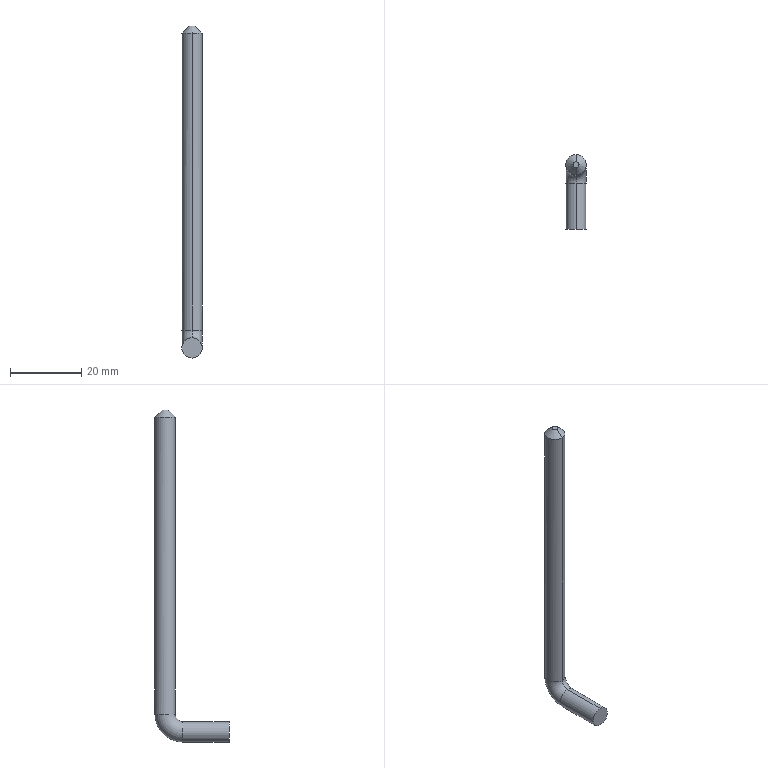Part | STEP file | RJWD-DY-0103_X2_53F367DC95E8_10 | 1 solid | 10 faces | box 5.7 x 20.85 x 93.35 mm | volume 2686 mm3 | cylinder 4 | cone 2 | plane 2 | torus 2 | commonest cylinder face diameters 5.7 x4
STEP:
#1=CARTESIAN_POINT('',(0.,0.,0.));
#2=DIRECTION('',(0.,0.,1.));
#3=DIRECTION('',(1.,0.,0.));
#4=AXIS2_PLACEMENT_3D('',#1,#2,#3);
#5=CARTESIAN_POINT('',(-506.773,5755.923,1751.394));
#6=VERTEX_POINT('',#5);
#7=CARTESIAN_POINT('',(-509.623,5753.073,1751.394));
#8=VERTEX_POINT('',#7);
#9=CARTESIAN_POINT('',(-506.773,5753.073,1751.394));
#10=DIRECTION('',(0.,0.,1.));
#11=DIRECTION('',(0.,1.,0.));
#12=AXIS2_PLACEMENT_3D('',#9,#10,#11);
#13=CIRCLE('',#12,2.85);
#14=CARTESIAN_POINT('',(-506.773,5753.073,1752.394));
#15=DIRECTION('',(0.,0.,-1.));
#16=DIRECTION('',(1.,0.,0.));
#17=AXIS2_PLACEMENT_3D('',#14,#15,#16);
#18=CONICAL_SURFACE('',#17,1.85,0.7854);
#19=CARTESIAN_POINT('',(4.712,1.));
#20=DIRECTION('',(-1.,0.));
#21=VECTOR('',#20,1.);
#22=LINE('',#19,#21);
#23=(GEOMETRIC_REPRESENTATION_CONTEXT(2)PARAMETRIC_REPRESENTATION_CONTEXT()REPRESENTATION_CONTEXT('',''));
#24=DEFINITIONAL_REPRESENTATION('',(#22),#23);
#25=PCURVE('',#18,#24);
#26=CARTESIAN_POINT('',(-506.773,5753.073,1753.394));
#27=DIRECTION('',(0.,0.,-1.));
#28=DIRECTION('',(0.,-1.,0.));
#29=AXIS2_PLACEMENT_3D('',#26,#27,#28);
#30=CYLINDRICAL_SURFACE('',#29,2.85);
#31=CARTESIAN_POINT('',(3.142,2.));
#32=DIRECTION('',(-1.,0.));
#33=VECTOR('',#32,1.);
#34=LINE('',#31,#33);
#35=(GEOMETRIC_REPRESENTATION_CONTEXT(2)PARAMETRIC_REPRESENTATION_CONTEXT()REPRESENTATION_CONTEXT('',''));
#36=DEFINITIONAL_REPRESENTATION('',(#34),#35);
#37=PCURVE('',#30,#36);
#38=SURFACE_CURVE('',#13,(#25,#37),.PCURVE_S1.);
#39=EDGE_CURVE('',#6,#8,#38,.T.);
#40=ORIENTED_EDGE('',*,*,#39,.T.);
#41=CARTESIAN_POINT('',(-506.773,5750.223,1751.394));
#42=VERTEX_POINT('',#41);
#43=CARTESIAN_POINT('',(-506.773,5753.073,1751.394));
#44=DIRECTION('',(0.,0.,1.));
#45=DIRECTION('',(-1.,0.,0.));
#46=AXIS2_PLACEMENT_3D('',#43,#44,#45);
#47=CIRCLE('',#46,2.85);
#48=CARTESIAN_POINT('',(3.142,1.));
#49=DIRECTION('',(-1.,0.));
#50=VECTOR('',#49,1.);
#51=LINE('',#48,#50);
#52=(GEOMETRIC_REPRESENTATION_CONTEXT(2)PARAMETRIC_REPRESENTATION_CONTEXT()REPRESENTATION_CONTEXT('',''));
#53=DEFINITIONAL_REPRESENTATION('',(#51),#52);
#54=PCURVE('',#18,#53);
#55=CARTESIAN_POINT('',(1.571,2.));
#56=DIRECTION('',(-1.,0.));
#57=VECTOR('',#56,1.);
#58=LINE('',#55,#57);
#59=(GEOMETRIC_REPRESENTATION_CONTEXT(2)PARAMETRIC_REPRESENTATION_CONTEXT()REPRESENTATION_CONTEXT('',''));
#60=DEFINITIONAL_REPRESENTATION('',(#58),#59);
#61=PCURVE('',#30,#60);
#62=SURFACE_CURVE('',#47,(#54,#61),.PCURVE_S1.);
#63=EDGE_CURVE('',#8,#42,#62,.T.);
#64=ORIENTED_EDGE('',*,*,#63,.T.);
#65=CARTESIAN_POINT('',(-506.773,5752.223,1753.394));
#66=VERTEX_POINT('',#65);
#67=CARTESIAN_POINT('',(-506.773,5750.223,1751.394));
#68=DIRECTION('',(0.,0.7071,0.7071));
#69=VECTOR('',#68,1.);
#70=LINE('',#67,#69);
#71=CARTESIAN_POINT('',(1.571,1.));
#72=DIRECTION('',(0.,-1.));
#73=VECTOR('',#72,1.);
#74=LINE('',#71,#73);
#75=(GEOMETRIC_REPRESENTATION_CONTEXT(2)PARAMETRIC_REPRESENTATION_CONTEXT()REPRESENTATION_CONTEXT('',''));
#76=DEFINITIONAL_REPRESENTATION('',(#74),#75);
#77=PCURVE('',#18,#76);
#78=CARTESIAN_POINT('',(-506.773,5753.073,1752.394));
#79=DIRECTION('',(0.,0.,-1.));
#80=DIRECTION('',(1.,0.,0.));
#81=AXIS2_PLACEMENT_3D('',#78,#79,#80);
#82=CONICAL_SURFACE('',#81,1.85,0.7854);
#83=CARTESIAN_POINT('',(7.854,1.));
#84=DIRECTION('',(0.,-1.));
#85=VECTOR('',#84,1.);
#86=LINE('',#83,#85);
#87=(GEOMETRIC_REPRESENTATION_CONTEXT(2)PARAMETRIC_REPRESENTATION_CONTEXT()REPRESENTATION_CONTEXT('',''));
#88=DEFINITIONAL_REPRESENTATION('',(#86),#87);
#89=PCURVE('',#82,#88);
#90=SURFACE_CURVE('',#70,(#77,#89),.PCURVE_S1.);
#91=EDGE_CURVE('',#42,#66,#90,.T.);
#92=ORIENTED_EDGE('',*,*,#91,.T.);
#93=CARTESIAN_POINT('',(-507.623,5753.073,1753.394));
#94=VERTEX_POINT('',#93);
#95=CARTESIAN_POINT('',(-506.773,5753.073,1753.394));
#96=DIRECTION('',(0.,0.,1.));
#97=DIRECTION('',(-1.,0.,0.));
#98=AXIS2_PLACEMENT_3D('',#95,#96,#97);
#99=CIRCLE('',#98,0.85);
#100=CARTESIAN_POINT('',(3.142,-1.));
#101=DIRECTION('',(-1.,0.));
#102=VECTOR('',#101,1.);
#103=LINE('',#100,#102);
#104=(GEOMETRIC_REPRESENTATION_CONTEXT(2)PARAMETRIC_REPRESENTATION_CONTEXT()REPRESENTATION_CONTEXT('',''));
#105=DEFINITIONAL_REPRESENTATION('',(#103),#104);
#106=PCURVE('',#18,#105);
#107=CARTESIAN_POINT('',(-506.773,5753.073,1753.394));
#108=DIRECTION('',(0.,0.,-1.));
#109=DIRECTION('',(0.,-1.,0.));
#110=AXIS2_PLACEMENT_3D('',#107,#108,#109);
#111=PLANE('',#110);
#112=CARTESIAN_POINT('',(0.,0.85));
#113=CARTESIAN_POINT('',(1.472,0.85));
#114=CARTESIAN_POINT('',(0.7361,-0.425));
#115=CARTESIAN_POINT('',(0.,-1.7));
#116=CARTESIAN_POINT('',(-0.7361,-0.425));
#117=CARTESIAN_POINT('',(-1.472,0.85));
#118=CARTESIAN_POINT('',(0.,0.85));
#119=(BOUNDED_CURVE()B_SPLINE_CURVE(2,(#112,#113,#114,#115,#116,#117,#118),.UNSPECIFIED.,.T.,.F.)B_SPLINE_CURVE_WITH_KNOTS((1,2,2,2,2,1),(-2.094,0.,2.094,4.189,6.283,8.378),.UNSPECIFIED.)CURVE()GEOMETRIC_REPRESENTATION_ITEM()RATIONAL_B_SPLINE_CURVE((1.,0.5,1.,0.5,1.,0.5,1.))REPRESENTATION_ITEM(''));
#120=(GEOMETRIC_REPRESENTATION_CONTEXT(2)PARAMETRIC_REPRESENTATION_CONTEXT()REPRESENTATION_CONTEXT('',''));
#121=DEFINITIONAL_REPRESENTATION('',(#119),#120);
#122=PCURVE('',#111,#121);
#123=SURFACE_CURVE('',#99,(#106,#122),.PCURVE_S1.);
#124=EDGE_CURVE('',#94,#66,#123,.T.);
#125=ORIENTED_EDGE('',*,*,#124,.F.);
#126=CARTESIAN_POINT('',(-506.773,5753.923,1753.394));
#127=VERTEX_POINT('',#126);
#128=CARTESIAN_POINT('',(-506.773,5753.073,1753.394));
#129=DIRECTION('',(0.,0.,1.));
#130=DIRECTION('',(0.,1.,0.));
#131=AXIS2_PLACEMENT_3D('',#128,#129,#130);
#132=CIRCLE('',#131,0.85);
#133=CARTESIAN_POINT('',(4.712,-1.));
#134=DIRECTION('',(-1.,0.));
#135=VECTOR('',#134,1.);
#136=LINE('',#133,#135);
#137=(GEOMETRIC_REPRESENTATION_CONTEXT(2)PARAMETRIC_REPRESENTATION_CONTEXT()REPRESENTATION_CONTEXT('',''));
#138=DEFINITIONAL_REPRESENTATION('',(#136),#137);
#139=PCURVE('',#18,#138);
#140=CARTESIAN_POINT('',(-0.85,0.));
#141=CARTESIAN_POINT('',(-0.85,1.472));
#142=CARTESIAN_POINT('',(0.425,0.7361));
#143=CARTESIAN_POINT('',(1.7,0.));
#144=CARTESIAN_POINT('',(0.425,-0.7361));
#145=CARTESIAN_POINT('',(-0.85,-1.472));
#146=CARTESIAN_POINT('',(-0.85,0.));
#147=(BOUNDED_CURVE()B_SPLINE_CURVE(2,(#140,#141,#142,#143,#144,#145,#146),.UNSPECIFIED.,.T.,.F.)B_SPLINE_CURVE_WITH_KNOTS((1,2,2,2,2,1),(-2.094,0.,2.094,4.189,6.283,8.378),.UNSPECIFIED.)CURVE()GEOMETRIC_REPRESENTATION_ITEM()RATIONAL_B_SPLINE_CURVE((1.,0.5,1.,0.5,1.,0.5,1.))REPRESENTATION_ITEM(''));
#148=(GEOMETRIC_REPRESENTATION_CONTEXT(2)PARAMETRIC_REPRESENTATION_CONTEXT()REPRESENTATION_CONTEXT('',''));
#149=DEFINITIONAL_REPRESENTATION('',(#147),#148);
#150=PCURVE('',#111,#149);
#151=SURFACE_CURVE('',#132,(#139,#150),.PCURVE_S1.);
#152=EDGE_CURVE('',#127,#94,#151,.T.);
#153=ORIENTED_EDGE('',*,*,#152,.F.);
#154=CARTESIAN_POINT('',(-506.773,5755.923,1751.394));
#155=DIRECTION('',(0.,-0.7071,0.7071));
#156=VECTOR('',#155,1.);
#157=LINE('',#154,#156);
#158=CARTESIAN_POINT('',(4.712,1.));
#159=DIRECTION('',(0.,-1.));
#160=VECTOR('',#159,1.);
#161=LINE('',#158,#160);
#162=(GEOMETRIC_REPRESENTATION_CONTEXT(2)PARAMETRIC_REPRESENTATION_CONTEXT()REPRESENTATION_CONTEXT('',''));
#163=DEFINITIONAL_REPRESENTATION('',(#161),#162);
#164=PCURVE('',#18,#163);
#165=CARTESIAN_POINT('',(4.712,1.));
#166=DIRECTION('',(0.,-1.));
#167=VECTOR('',#166,1.);
#168=LINE('',#165,#167);
#169=(GEOMETRIC_REPRESENTATION_CONTEXT(2)PARAMETRIC_REPRESENTATION_CONTEXT()REPRESENTATION_CONTEXT('',''));
#170=DEFINITIONAL_REPRESENTATION('',(#168),#169);
#171=PCURVE('',#82,#170);
#172=SURFACE_CURVE('',#157,(#164,#171),.PCURVE_S1.);
#173=EDGE_CURVE('',#6,#127,#172,.T.);
#174=ORIENTED_EDGE('',*,*,#173,.F.);
#175=EDGE_LOOP('',(#40,#64,#92,#125,#153,#174));
#176=FACE_BOUND('',#175,.T.);
#177=ADVANCED_FACE('',(#176),#18,.T.);
#178=CARTESIAN_POINT('',(-503.923,5753.073,1751.394));
#179=VERTEX_POINT('',#178);
#180=CARTESIAN_POINT('',(-506.773,5753.073,1751.394));
#181=DIRECTION('',(0.,0.,1.));
#182=DIRECTION('',(0.,-1.,0.));
#183=AXIS2_PLACEMENT_3D('',#180,#181,#182);
#184=CIRCLE('',#183,2.85);
#185=CARTESIAN_POINT('',(7.854,1.));
#186=DIRECTION('',(-1.,0.));
#187=VECTOR('',#186,1.);
#188=LINE('',#185,#187);
#189=(GEOMETRIC_REPRESENTATION_CONTEXT(2)PARAMETRIC_REPRESENTATION_CONTEXT()REPRESENTATION_CONTEXT('',''));
#190=DEFINITIONAL_REPRESENTATION('',(#188),#189);
#191=PCURVE('',#82,#190);
#192=CARTESIAN_POINT('',(-506.773,5753.073,1753.394));
#193=DIRECTION('',(0.,0.,-1.));
#194=DIRECTION('',(0.,-1.,0.));
#195=AXIS2_PLACEMENT_3D('',#192,#193,#194);
#196=CYLINDRICAL_SURFACE('',#195,2.85);
#197=CARTESIAN_POINT('',(6.283,2.));
#198=DIRECTION('',(-1.,0.));
#199=VECTOR('',#198,1.);
#200=LINE('',#197,#199);
#201=(GEOMETRIC_REPRESENTATION_CONTEXT(2)PARAMETRIC_REPRESENTATION_CONTEXT()REPRESENTATION_CONTEXT('',''));
#202=DEFINITIONAL_REPRESENTATION('',(#200),#201);
#203=PCURVE('',#196,#202);
#204=SURFACE_CURVE('',#184,(#191,#203),.PCURVE_S1.);
#205=EDGE_CURVE('',#42,#179,#204,.T.);
#206=ORIENTED_EDGE('',*,*,#205,.T.);
#207=CARTESIAN_POINT('',(-506.773,5753.073,1751.394));
#208=DIRECTION('',(0.,0.,1.));
#209=DIRECTION('',(1.,0.,0.));
#210=AXIS2_PLACEMENT_3D('',#207,#208,#209);
#211=CIRCLE('',#210,2.85);
#212=CARTESIAN_POINT('',(6.283,1.));
#213=DIRECTION('',(-1.,0.));
#214=VECTOR('',#213,1.);
#215=LINE('',#212,#214);
#216=(GEOMETRIC_REPRESENTATION_CONTEXT(2)PARAMETRIC_REPRESENTATION_CONTEXT()REPRESENTATION_CONTEXT('',''));
#217=DEFINITIONAL_REPRESENTATION('',(#215),#216);
#218=PCURVE('',#82,#217);
#219=CARTESIAN_POINT('',(4.712,2.));
#220=DIRECTION('',(-1.,0.));
#221=VECTOR('',#220,1.);
#222=LINE('',#219,#221);
#223=(GEOMETRIC_REPRESENTATION_CONTEXT(2)PARAMETRIC_REPRESENTATION_CONTEXT()REPRESENTATION_CONTEXT('',''));
#224=DEFINITIONAL_REPRESENTATION('',(#222),#223);
#225=PCURVE('',#196,#224);
#226=SURFACE_CURVE('',#211,(#218,#225),.PCURVE_S1.);
#227=EDGE_CURVE('',#179,#6,#226,.T.);
#228=ORIENTED_EDGE('',*,*,#227,.T.);
#229=ORIENTED_EDGE('',*,*,#173,.T.);
#230=CARTESIAN_POINT('',(-505.923,5753.073,1753.394));
#231=VERTEX_POINT('',#230);
#232=CARTESIAN_POINT('',(-506.773,5753.073,1753.394));
#233=DIRECTION('',(0.,0.,1.));
#234=DIRECTION('',(1.,0.,0.));
#235=AXIS2_PLACEMENT_3D('',#232,#233,#234);
#236=CIRCLE('',#235,0.85);
#237=CARTESIAN_POINT('',(6.283,-1.));
#238=DIRECTION('',(-1.,0.));
#239=VECTOR('',#238,1.);
#240=LINE('',#237,#239);
#241=(GEOMETRIC_REPRESENTATION_CONTEXT(2)PARAMETRIC_REPRESENTATION_CONTEXT()REPRESENTATION_CONTEXT('',''));
#242=DEFINITIONAL_REPRESENTATION('',(#240),#241);
#243=PCURVE('',#82,#242);
#244=CARTESIAN_POINT('',(0.,-0.85));
#245=CARTESIAN_POINT('',(-1.472,-0.85));
#246=CARTESIAN_POINT('',(-0.7361,0.425));
#247=CARTESIAN_POINT('',(0.,1.7));
#248=CARTESIAN_POINT('',(0.7361,0.425));
#249=CARTESIAN_POINT('',(1.472,-0.85));
#250=CARTESIAN_POINT('',(0.,-0.85));
#251=(BOUNDED_CURVE()B_SPLINE_CURVE(2,(#244,#245,#246,#247,#248,#249,#250),.UNSPECIFIED.,.T.,.F.)B_SPLINE_CURVE_WITH_KNOTS((1,2,2,2,2,1),(-2.094,0.,2.094,4.189,6.283,8.378),.UNSPECIFIED.)CURVE()GEOMETRIC_REPRESENTATION_ITEM()RATIONAL_B_SPLINE_CURVE((1.,0.5,1.,0.5,1.,0.5,1.))REPRESENTATION_ITEM(''));
#252=(GEOMETRIC_REPRESENTATION_CONTEXT(2)PARAMETRIC_REPRESENTATION_CONTEXT()REPRESENTATION_CONTEXT('',''));
#253=DEFINITIONAL_REPRESENTATION('',(#251),#252);
#254=PCURVE('',#111,#253);
#255=SURFACE_CURVE('',#236,(#243,#254),.PCURVE_S1.);
#256=EDGE_CURVE('',#231,#127,#255,.T.);
#257=ORIENTED_EDGE('',*,*,#256,.F.);
#258=CARTESIAN_POINT('',(-506.773,5753.073,1753.394));
#259=DIRECTION('',(0.,0.,1.));
#260=DIRECTION('',(0.,-1.,0.));
#261=AXIS2_PLACEMENT_3D('',#258,#259,#260);
#262=CIRCLE('',#261,0.85);
#263=CARTESIAN_POINT('',(7.854,-1.));
#264=DIRECTION('',(-1.,0.));
#265=VECTOR('',#264,1.);
#266=LINE('',#263,#265);
#267=(GEOMETRIC_REPRESENTATION_CONTEXT(2)PARAMETRIC_REPRESENTATION_CONTEXT()REPRESENTATION_CONTEXT('',''));
#268=DEFINITIONAL_REPRESENTATION('',(#266),#267);
#269=PCURVE('',#82,#268);
#270=CARTESIAN_POINT('',(0.85,0.));
#271=CARTESIAN_POINT('',(0.85,-1.472));
#272=CARTESIAN_POINT('',(-0.425,-0.7361));
#273=CARTESIAN_POINT('',(-1.7,0.));
#274=CARTESIAN_POINT('',(-0.425,0.7361));
#275=CARTESIAN_POINT('',(0.85,1.472));
#276=CARTESIAN_POINT('',(0.85,0.));
#277=(BOUNDED_CURVE()B_SPLINE_CURVE(2,(#270,#271,#272,#273,#274,#275,#276),.UNSPECIFIED.,.T.,.F.)B_SPLINE_CURVE_WITH_KNOTS((1,2,2,2,2,1),(-2.094,0.,2.094,4.189,6.283,8.378),.UNSPECIFIED.)CURVE()GEOMETRIC_REPRESENTATION_ITEM()RATIONAL_B_SPLINE_CURVE((1.,0.5,1.,0.5,1.,0.5,1.))REPRESENTATION_ITEM(''));
#278=(GEOMETRIC_REPRESENTATION_CONTEXT(2)PARAMETRIC_REPRESENTATION_CONTEXT()REPRESENTATION_CONTEXT('',''));
#279=DEFINITIONAL_REPRESENTATION('',(#277),#278);
#280=PCURVE('',#111,#279);
#281=SURFACE_CURVE('',#262,(#269,#280),.PCURVE_S1.);
#282=EDGE_CURVE('',#66,#231,#281,.T.);
#283=ORIENTED_EDGE('',*,*,#282,.F.);
#284=ORIENTED_EDGE('',*,*,#91,.F.);
#285=EDGE_LOOP('',(#206,#228,#229,#257,#283,#284));
#286=FACE_BOUND('',#285,.T.);
#287=ADVANCED_FACE('',(#286),#82,.T.);
#288=ORIENTED_EDGE('',*,*,#152,.F.);
#289=ORIENTED_EDGE('',*,*,#256,.F.);
#290=ORIENTED_EDGE('',*,*,#282,.F.);
#291=ORIENTED_EDGE('',*,*,#124,.F.);
#292=EDGE_LOOP('',(#288,#289,#290,#291));
#293=FACE_BOUND('',#292,.F.);
#294=ADVANCED_FACE('',(#293),#111,.F.);
#295=ORIENTED_EDGE('',*,*,#205,.F.);
#296=CARTESIAN_POINT('',(-506.773,5750.223,1667.894));
#297=VERTEX_POINT('',#296);
#298=CARTESIAN_POINT('',(-506.773,5750.223,1667.894));
#299=DIRECTION('',(0.,0.,1.));
#300=VECTOR('',#299,1.);
#301=LINE('',#298,#300);
#302=CARTESIAN_POINT('',(6.283,85.5));
#303=DIRECTION('',(0.,-1.));
#304=VECTOR('',#303,1.);
#305=LINE('',#302,#304);
#306=(GEOMETRIC_REPRESENTATION_CONTEXT(2)PARAMETRIC_REPRESENTATION_CONTEXT()REPRESENTATION_CONTEXT('',''));
#307=DEFINITIONAL_REPRESENTATION('',(#305),#306);
#308=PCURVE('',#196,#307);
#309=CARTESIAN_POINT('',(0.,85.5));
#310=DIRECTION('',(0.,-1.));
#311=VECTOR('',#310,1.);
#312=LINE('',#309,#311);
#313=(GEOMETRIC_REPRESENTATION_CONTEXT(2)PARAMETRIC_REPRESENTATION_CONTEXT()REPRESENTATION_CONTEXT('',''));
#314=DEFINITIONAL_REPRESENTATION('',(#312),#313);
#315=PCURVE('',#30,#314);
#316=SURFACE_CURVE('',#301,(#308,#315),.PCURVE_S1.);
#317=EDGE_CURVE('',#297,#42,#316,.T.);
#318=ORIENTED_EDGE('',*,*,#317,.F.);
#319=CARTESIAN_POINT('',(-506.773,5755.923,1667.894));
#320=VERTEX_POINT('',#319);
#321=CARTESIAN_POINT('',(-506.773,5753.073,1667.894));
#322=DIRECTION('',(0.,0.,-1.));
#323=DIRECTION('',(0.,1.,0.));
#324=AXIS2_PLACEMENT_3D('',#321,#322,#323);
#325=CIRCLE('',#324,2.85);
#326=CARTESIAN_POINT('',(3.142,85.5));
#327=DIRECTION('',(1.,0.));
#328=VECTOR('',#327,1.);
#329=LINE('',#326,#328);
#330=(GEOMETRIC_REPRESENTATION_CONTEXT(2)PARAMETRIC_REPRESENTATION_CONTEXT()REPRESENTATION_CONTEXT('',''));
#331=DEFINITIONAL_REPRESENTATION('',(#329),#330);
#332=PCURVE('',#196,#331);
#333=CARTESIAN_POINT('',(-506.773,5748.073,1667.894));
#334=DIRECTION('',(-1.,0.,0.));
#335=DIRECTION('',(0.,1.,0.));
#336=AXIS2_PLACEMENT_3D('',#333,#334,#335);
#337=TOROIDAL_SURFACE('',#336,5.,2.85);
#338=CARTESIAN_POINT('',(0.,6.283));
#339=DIRECTION('',(0.,-1.));
#340=VECTOR('',#339,1.);
#341=LINE('',#338,#340);
#342=(GEOMETRIC_REPRESENTATION_CONTEXT(2)PARAMETRIC_REPRESENTATION_CONTEXT()REPRESENTATION_CONTEXT('',''));
#343=DEFINITIONAL_REPRESENTATION('',(#341),#342);
#344=PCURVE('',#337,#343);
#345=SURFACE_CURVE('',#325,(#332,#344),.PCURVE_S1.);
#346=EDGE_CURVE('',#320,#297,#345,.T.);
#347=ORIENTED_EDGE('',*,*,#346,.F.);
#348=CARTESIAN_POINT('',(-506.773,5755.923,1667.894));
#349=DIRECTION('',(0.,0.,1.));
#350=VECTOR('',#349,1.);
#351=LINE('',#348,#350);
#352=CARTESIAN_POINT('',(3.142,85.5));
#353=DIRECTION('',(0.,-1.));
#354=VECTOR('',#353,1.);
#355=LINE('',#352,#354);
#356=(GEOMETRIC_REPRESENTATION_CONTEXT(2)PARAMETRIC_REPRESENTATION_CONTEXT()REPRESENTATION_CONTEXT('',''));
#357=DEFINITIONAL_REPRESENTATION('',(#355),#356);
#358=PCURVE('',#196,#357);
#359=CARTESIAN_POINT('',(3.142,85.5));
#360=DIRECTION('',(0.,-1.));
#361=VECTOR('',#360,1.);
#362=LINE('',#359,#361);
#363=(GEOMETRIC_REPRESENTATION_CONTEXT(2)PARAMETRIC_REPRESENTATION_CONTEXT()REPRESENTATION_CONTEXT('',''));
#364=DEFINITIONAL_REPRESENTATION('',(#362),#363);
#365=PCURVE('',#30,#364);
#366=SURFACE_CURVE('',#351,(#358,#365),.PCURVE_S1.);
#367=EDGE_CURVE('',#320,#6,#366,.T.);
#368=ORIENTED_EDGE('',*,*,#367,.T.);
#369=ORIENTED_EDGE('',*,*,#227,.F.);
#370=EDGE_LOOP('',(#295,#318,#347,#368,#369));
#371=FACE_BOUND('',#370,.T.);
#372=ADVANCED_FACE('',(#371),#196,.T.);
#373=ORIENTED_EDGE('',*,*,#317,.T.);
#374=ORIENTED_EDGE('',*,*,#63,.F.);
#375=ORIENTED_EDGE('',*,*,#39,.F.);
#376=ORIENTED_EDGE('',*,*,#367,.F.);
#377=CARTESIAN_POINT('',(-506.773,5753.073,1667.894));
#378=DIRECTION('',(0.,0.,-1.));
#379=DIRECTION('',(0.,-1.,0.));
#380=AXIS2_PLACEMENT_3D('',#377,#378,#379);
#381=CIRCLE('',#380,2.85);
#382=CARTESIAN_POINT('',(0.,85.5));
#383=DIRECTION('',(1.,0.));
#384=VECTOR('',#383,1.);
#385=LINE('',#382,#384);
#386=(GEOMETRIC_REPRESENTATION_CONTEXT(2)PARAMETRIC_REPRESENTATION_CONTEXT()REPRESENTATION_CONTEXT('',''));
#387=DEFINITIONAL_REPRESENTATION('',(#385),#386);
#388=PCURVE('',#30,#387);
#389=CARTESIAN_POINT('',(-506.773,5748.073,1667.894));
#390=DIRECTION('',(-1.,0.,0.));
#391=DIRECTION('',(0.,1.,0.));
#392=AXIS2_PLACEMENT_3D('',#389,#390,#391);
#393=TOROIDAL_SURFACE('',#392,5.,2.85);
#394=CARTESIAN_POINT('',(0.,3.142));
#395=DIRECTION('',(0.,-1.));
#396=VECTOR('',#395,1.);
#397=LINE('',#394,#396);
#398=(GEOMETRIC_REPRESENTATION_CONTEXT(2)PARAMETRIC_REPRESENTATION_CONTEXT()REPRESENTATION_CONTEXT('',''));
#399=DEFINITIONAL_REPRESENTATION('',(#397),#398);
#400=PCURVE('',#393,#399);
#401=SURFACE_CURVE('',#381,(#388,#400),.PCURVE_S1.);
#402=EDGE_CURVE('',#297,#320,#401,.T.);
#403=ORIENTED_EDGE('',*,*,#402,.F.);
#404=EDGE_LOOP('',(#373,#374,#375,#376,#403));
#405=FACE_BOUND('',#404,.T.);
#406=ADVANCED_FACE('',(#405),#30,.T.);
#407=CARTESIAN_POINT('',(-506.773,5748.073,1660.044));
#408=VERTEX_POINT('',#407);
#409=CARTESIAN_POINT('',(-506.773,5748.073,1665.744));
#410=VERTEX_POINT('',#409);
#411=CARTESIAN_POINT('',(-506.773,5748.073,1662.894));
#412=DIRECTION('',(0.,1.,0.));
#413=DIRECTION('',(0.,0.,-1.));
#414=AXIS2_PLACEMENT_3D('',#411,#412,#413);
#415=CIRCLE('',#414,2.85);
#416=CARTESIAN_POINT('',(1.571,0.));
#417=DIRECTION('',(0.,1.));
#418=VECTOR('',#417,1.);
#419=LINE('',#416,#418);
#420=(GEOMETRIC_REPRESENTATION_CONTEXT(2)PARAMETRIC_REPRESENTATION_CONTEXT()REPRESENTATION_CONTEXT('',''));
#421=DEFINITIONAL_REPRESENTATION('',(#419),#420);
#422=PCURVE('',#393,#421);
#423=CARTESIAN_POINT('',(-506.773,5748.073,1662.894));
#424=DIRECTION('',(0.,-1.,0.));
#425=DIRECTION('',(0.,0.,1.));
#426=AXIS2_PLACEMENT_3D('',#423,#424,#425);
#427=CYLINDRICAL_SURFACE('',#426,2.85);
#428=CARTESIAN_POINT('',(3.142,0.));
#429=DIRECTION('',(-1.,0.));
#430=VECTOR('',#429,1.);
#431=LINE('',#428,#430);
#432=(GEOMETRIC_REPRESENTATION_CONTEXT(2)PARAMETRIC_REPRESENTATION_CONTEXT()REPRESENTATION_CONTEXT('',''));
#433=DEFINITIONAL_REPRESENTATION('',(#431),#432);
#434=PCURVE('',#427,#433);
#435=SURFACE_CURVE('',#415,(#422,#434),.PCURVE_S1.);
#436=EDGE_CURVE('',#408,#410,#435,.T.);
#437=ORIENTED_EDGE('',*,*,#436,.T.);
#438=CARTESIAN_POINT('',(-506.773,5748.073,1667.894));
#439=DIRECTION('',(1.,0.,0.));
#440=DIRECTION('',(0.,0.,-1.));
#441=AXIS2_PLACEMENT_3D('',#438,#439,#440);
#442=CIRCLE('',#441,2.15);
#443=CARTESIAN_POINT('',(1.571,3.142));
#444=DIRECTION('',(-1.,0.));
#445=VECTOR('',#444,1.);
#446=LINE('',#443,#445);
#447=(GEOMETRIC_REPRESENTATION_CONTEXT(2)PARAMETRIC_REPRESENTATION_CONTEXT()REPRESENTATION_CONTEXT('',''));
#448=DEFINITIONAL_REPRESENTATION('',(#446),#447);
#449=PCURVE('',#393,#448);
#450=CARTESIAN_POINT('',(1.571,3.142));
#451=DIRECTION('',(-1.,0.));
#452=VECTOR('',#451,1.);
#453=LINE('',#450,#452);
#454=(GEOMETRIC_REPRESENTATION_CONTEXT(2)PARAMETRIC_REPRESENTATION_CONTEXT()REPRESENTATION_CONTEXT('',''));
#455=DEFINITIONAL_REPRESENTATION('',(#453),#454);
#456=PCURVE('',#337,#455);
#457=SURFACE_CURVE('',#442,(#449,#456),.PCURVE_S1.);
#458=EDGE_CURVE('',#410,#297,#457,.T.);
#459=ORIENTED_EDGE('',*,*,#458,.T.);
#460=ORIENTED_EDGE('',*,*,#402,.T.);
#461=CARTESIAN_POINT('',(-506.773,5748.073,1667.894));
#462=DIRECTION('',(1.,0.,0.));
#463=DIRECTION('',(0.,0.,-1.));
#464=AXIS2_PLACEMENT_3D('',#461,#462,#463);
#465=CIRCLE('',#464,7.85);
#466=CARTESIAN_POINT('',(1.571,0.));
#467=DIRECTION('',(-1.,0.));
#468=VECTOR('',#467,1.);
#469=LINE('',#466,#468);
#470=(GEOMETRIC_REPRESENTATION_CONTEXT(2)PARAMETRIC_REPRESENTATION_CONTEXT()REPRESENTATION_CONTEXT('',''));
#471=DEFINITIONAL_REPRESENTATION('',(#469),#470);
#472=PCURVE('',#393,#471);
#473=CARTESIAN_POINT('',(1.571,6.283));
#474=DIRECTION('',(-1.,0.));
#475=VECTOR('',#474,1.);
#476=LINE('',#473,#475);
#477=(GEOMETRIC_REPRESENTATION_CONTEXT(2)PARAMETRIC_REPRESENTATION_CONTEXT()REPRESENTATION_CONTEXT('',''));
#478=DEFINITIONAL_REPRESENTATION('',(#476),#477);
#479=PCURVE('',#337,#478);
#480=SURFACE_CURVE('',#465,(#472,#479),.PCURVE_S1.);
#481=EDGE_CURVE('',#408,#320,#480,.T.);
#482=ORIENTED_EDGE('',*,*,#481,.F.);
#483=EDGE_LOOP('',(#437,#459,#460,#482));
#484=FACE_BOUND('',#483,.T.);
#485=ADVANCED_FACE('',(#484),#393,.T.);
#486=CARTESIAN_POINT('',(-506.773,5748.073,1662.894));
#487=DIRECTION('',(0.,1.,0.));
#488=DIRECTION('',(0.,0.,1.));
#489=AXIS2_PLACEMENT_3D('',#486,#487,#488);
#490=CIRCLE('',#489,2.85);
#491=CARTESIAN_POINT('',(1.571,3.142));
#492=DIRECTION('',(0.,1.));
#493=VECTOR('',#492,1.);
#494=LINE('',#491,#493);
#495=(GEOMETRIC_REPRESENTATION_CONTEXT(2)PARAMETRIC_REPRESENTATION_CONTEXT()REPRESENTATION_CONTEXT('',''));
#496=DEFINITIONAL_REPRESENTATION('',(#494),#495);
#497=PCURVE('',#337,#496);
#498=CARTESIAN_POINT('',(-506.773,5748.073,1662.894));
#499=DIRECTION('',(0.,-1.,0.));
#500=DIRECTION('',(0.,0.,1.));
#501=AXIS2_PLACEMENT_3D('',#498,#499,#500);
#502=CYLINDRICAL_SURFACE('',#501,2.85);
#503=CARTESIAN_POINT('',(6.283,0.));
#504=DIRECTION('',(-1.,0.));
#505=VECTOR('',#504,1.);
#506=LINE('',#503,#505);
#507=(GEOMETRIC_REPRESENTATION_CONTEXT(2)PARAMETRIC_REPRESENTATION_CONTEXT()REPRESENTATION_CONTEXT('',''));
#508=DEFINITIONAL_REPRESENTATION('',(#506),#507);
#509=PCURVE('',#502,#508);
#510=SURFACE_CURVE('',#490,(#497,#509),.PCURVE_S1.);
#511=EDGE_CURVE('',#410,#408,#510,.T.);
#512=ORIENTED_EDGE('',*,*,#511,.T.);
#513=ORIENTED_EDGE('',*,*,#481,.T.);
#514=ORIENTED_EDGE('',*,*,#346,.T.);
#515=ORIENTED_EDGE('',*,*,#458,.F.);
#516=EDGE_LOOP('',(#512,#513,#514,#515));
#517=FACE_BOUND('',#516,.T.);
#518=ADVANCED_FACE('',(#517),#337,.T.);
#519=CARTESIAN_POINT('',(-506.773,5735.073,1660.044));
#520=VERTEX_POINT('',#519);
#521=CARTESIAN_POINT('',(-506.773,5735.073,1665.744));
#522=VERTEX_POINT('',#521);
#523=CARTESIAN_POINT('',(-506.773,5735.073,1662.894));
#524=DIRECTION('',(0.,-1.,0.));
#525=DIRECTION('',(0.,0.,-1.));
#526=AXIS2_PLACEMENT_3D('',#523,#524,#525);
#527=CIRCLE('',#526,2.85);
#528=CARTESIAN_POINT('',(3.142,13.));
#529=DIRECTION('',(1.,0.));
#530=VECTOR('',#529,1.);
#531=LINE('',#528,#530);
#532=(GEOMETRIC_REPRESENTATION_CONTEXT(2)PARAMETRIC_REPRESENTATION_CONTEXT()REPRESENTATION_CONTEXT('',''));
#533=DEFINITIONAL_REPRESENTATION('',(#531),#532);
#534=PCURVE('',#502,#533);
#535=CARTESIAN_POINT('',(-506.773,5735.073,1662.894));
#536=DIRECTION('',(0.,-1.,0.));
#537=DIRECTION('',(0.,0.,1.));
#538=AXIS2_PLACEMENT_3D('',#535,#536,#537);
#539=PLANE('',#538);
#540=CARTESIAN_POINT('',(0.,0.));
#541=DIRECTION('',(-1.,0.));
#542=AXIS2_PLACEMENT_2D('',#540,#541);
#543=CIRCLE('',#542,2.85);
#544=(GEOMETRIC_REPRESENTATION_CONTEXT(2)PARAMETRIC_REPRESENTATION_CONTEXT()REPRESENTATION_CONTEXT('',''));
#545=DEFINITIONAL_REPRESENTATION('',(#543),#544);
#546=PCURVE('',#539,#545);
#547=SURFACE_CURVE('',#527,(#534,#546),.PCURVE_S1.);
#548=EDGE_CURVE('',#520,#522,#547,.T.);
#549=ORIENTED_EDGE('',*,*,#548,.F.);
#550=CARTESIAN_POINT('',(-506.773,5748.073,1660.044));
#551=DIRECTION('',(0.,-1.,0.));
#552=VECTOR('',#551,1.);
#553=LINE('',#550,#552);
#554=CARTESIAN_POINT('',(3.142,0.));
#555=DIRECTION('',(0.,1.));
#556=VECTOR('',#555,1.);
#557=LINE('',#554,#556);
#558=(GEOMETRIC_REPRESENTATION_CONTEXT(2)PARAMETRIC_REPRESENTATION_CONTEXT()REPRESENTATION_CONTEXT('',''));
#559=DEFINITIONAL_REPRESENTATION('',(#557),#558);
#560=PCURVE('',#502,#559);
#561=CARTESIAN_POINT('',(3.142,0.));
#562=DIRECTION('',(0.,1.));
#563=VECTOR('',#562,1.);
#564=LINE('',#561,#563);
#565=(GEOMETRIC_REPRESENTATION_CONTEXT(2)PARAMETRIC_REPRESENTATION_CONTEXT()REPRESENTATION_CONTEXT('',''));
#566=DEFINITIONAL_REPRESENTATION('',(#564),#565);
#567=PCURVE('',#427,#566);
#568=SURFACE_CURVE('',#553,(#560,#567),.PCURVE_S1.);
#569=EDGE_CURVE('',#408,#520,#568,.T.);
#570=ORIENTED_EDGE('',*,*,#569,.F.);
#571=ORIENTED_EDGE('',*,*,#511,.F.);
#572=CARTESIAN_POINT('',(-506.773,5748.073,1665.744));
#573=DIRECTION('',(0.,-1.,0.));
#574=VECTOR('',#573,1.);
#575=LINE('',#572,#574);
#576=CARTESIAN_POINT('',(6.283,0.));
#577=DIRECTION('',(0.,1.));
#578=VECTOR('',#577,1.);
#579=LINE('',#576,#578);
#580=(GEOMETRIC_REPRESENTATION_CONTEXT(2)PARAMETRIC_REPRESENTATION_CONTEXT()REPRESENTATION_CONTEXT('',''));
#581=DEFINITIONAL_REPRESENTATION('',(#579),#580);
#582=PCURVE('',#502,#581);
#583=CARTESIAN_POINT('',(0.,0.));
#584=DIRECTION('',(0.,1.));
#585=VECTOR('',#584,1.);
#586=LINE('',#583,#585);
#587=(GEOMETRIC_REPRESENTATION_CONTEXT(2)PARAMETRIC_REPRESENTATION_CONTEXT()REPRESENTATION_CONTEXT('',''));
#588=DEFINITIONAL_REPRESENTATION('',(#586),#587);
#589=PCURVE('',#427,#588);
#590=SURFACE_CURVE('',#575,(#582,#589),.PCURVE_S1.);
#591=EDGE_CURVE('',#410,#522,#590,.T.);
#592=ORIENTED_EDGE('',*,*,#591,.T.);
#593=EDGE_LOOP('',(#549,#570,#571,#592));
#594=FACE_BOUND('',#593,.T.);
#595=ADVANCED_FACE('',(#594),#502,.T.);
#596=CARTESIAN_POINT('',(-506.773,5735.073,1662.894));
#597=DIRECTION('',(0.,-1.,0.));
#598=DIRECTION('',(0.,0.,1.));
#599=AXIS2_PLACEMENT_3D('',#596,#597,#598);
#600=CIRCLE('',#599,2.85);
#601=CARTESIAN_POINT('',(0.,13.));
#602=DIRECTION('',(1.,0.));
#603=VECTOR('',#602,1.);
#604=LINE('',#601,#603);
#605=(GEOMETRIC_REPRESENTATION_CONTEXT(2)PARAMETRIC_REPRESENTATION_CONTEXT()REPRESENTATION_CONTEXT('',''));
#606=DEFINITIONAL_REPRESENTATION('',(#604),#605);
#607=PCURVE('',#427,#606);
#608=CARTESIAN_POINT('',(0.,0.));
#609=DIRECTION('',(1.,0.));
#610=AXIS2_PLACEMENT_2D('',#608,#609);
#611=CIRCLE('',#610,2.85);
#612=(GEOMETRIC_REPRESENTATION_CONTEXT(2)PARAMETRIC_REPRESENTATION_CONTEXT()REPRESENTATION_CONTEXT('',''));
#613=DEFINITIONAL_REPRESENTATION('',(#611),#612);
#614=PCURVE('',#539,#613);
#615=SURFACE_CURVE('',#600,(#607,#614),.PCURVE_S1.);
#616=EDGE_CURVE('',#522,#520,#615,.T.);
#617=ORIENTED_EDGE('',*,*,#616,.F.);
#618=ORIENTED_EDGE('',*,*,#591,.F.);
#619=ORIENTED_EDGE('',*,*,#436,.F.);
#620=ORIENTED_EDGE('',*,*,#569,.T.);
#621=EDGE_LOOP('',(#617,#618,#619,#620));
#622=FACE_BOUND('',#621,.T.);
#623=ADVANCED_FACE('',(#622),#427,.T.);
#624=ORIENTED_EDGE('',*,*,#616,.F.);
#625=ORIENTED_EDGE('',*,*,#548,.F.);
#626=EDGE_LOOP('',(#624,#625));
#627=FACE_BOUND('',#626,.F.);
#628=ADVANCED_FACE('',(#627),#539,.T.);
#629=CLOSED_SHELL('',(#177,#287,#294,#372,#406,#485,#518,#595,#623,#628));
#630=MANIFOLD_SOLID_BREP('',#629);
#631=(LENGTH_UNIT()NAMED_UNIT(*)SI_UNIT(.MILLI.,.METRE.));
#632=UNCERTAINTY_MEASURE_WITH_UNIT(LENGTH_MEASURE(0.0000001),#631,'','');
#633=(NAMED_UNIT(*)PLANE_ANGLE_UNIT()SI_UNIT($,.RADIAN.));
#634=(NAMED_UNIT(*)SI_UNIT($,.STERADIAN.)SOLID_ANGLE_UNIT());
#635=(GEOMETRIC_REPRESENTATION_CONTEXT(3)GLOBAL_UNCERTAINTY_ASSIGNED_CONTEXT((#632))GLOBAL_UNIT_ASSIGNED_CONTEXT((#631,#633,#634))REPRESENTATION_CONTEXT('',''));
#636=ADVANCED_BREP_SHAPE_REPRESENTATION('',(#4,#630),#635);